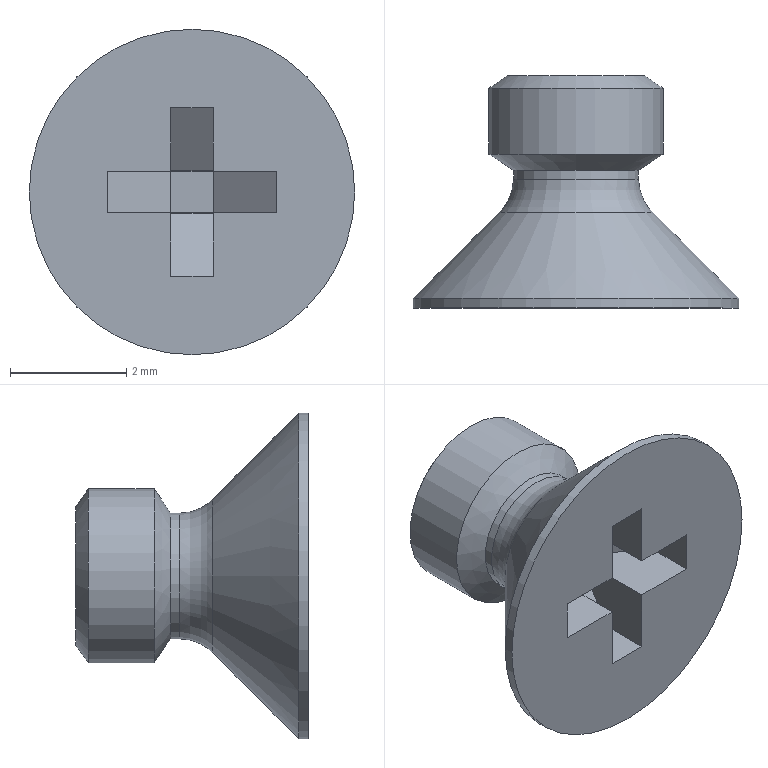Part | STEP file | Senkschraube_DIN_965_M3x4 | 1 solid | 26 faces | box 5.6 x 4 x 5.6 mm | volume 33.649 mm3 | plane 19 | cylinder 3 | cone 3 | torus 1 | commonest cylinder face diameters 2.161 x1 3 x1 5.6 x1